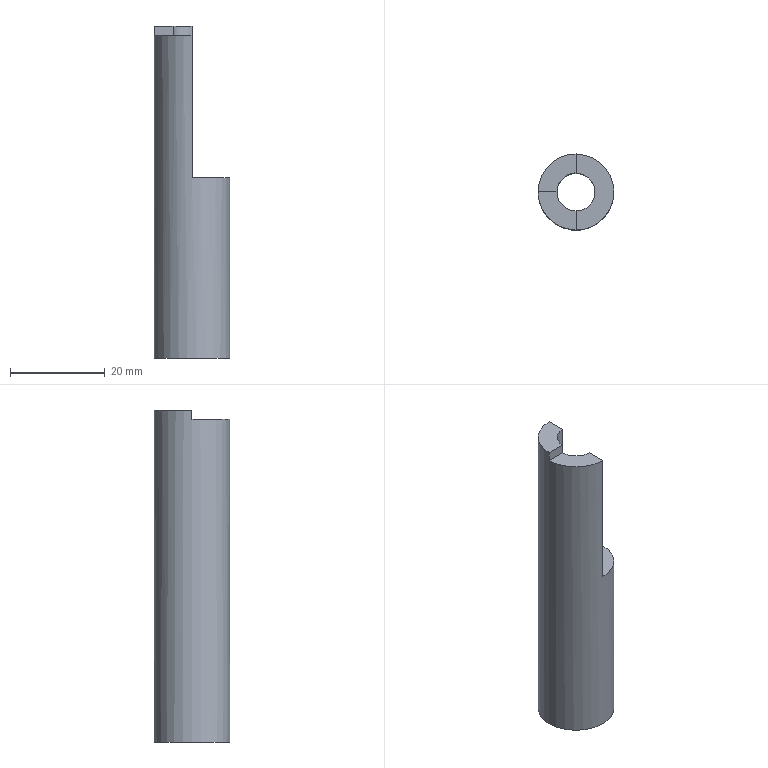Part | NX | features solid 2 | 1 solid | 9 faces | box 16 x 16 x 70 mm | volume 8068 mm3 | plane 7 | cylinder 2 | commonest cylinder face diameters 8 x1 16 x1
STEP:
#1=CARTESIAN_POINT('',(158.,4.,-34.5));
#2=VERTEX_POINT('',#1);
#3=CARTESIAN_POINT('',(158.,8.,-34.5));
#4=VERTEX_POINT('',#3);
#5=CARTESIAN_POINT('',(158.,0.000000002,-34.5));
#6=DIRECTION('',(0.,-1.,0.));
#7=VECTOR('',#6,1000.);
#8=LINE('',#5,#7);
#9=EDGE_CURVE('',#2,#4,#8,.F.);
#10=ORIENTED_EDGE('',*,*,#9,.F.);
#11=CARTESIAN_POINT('',(158.,-4.,-34.5));
#12=VERTEX_POINT('',#11);
#13=CARTESIAN_POINT('',(158.,0.000000002,-34.5));
#14=DIRECTION('',(0.,0.,-1.));
#15=DIRECTION('',(-1.,0.,0.));
#16=AXIS2_PLACEMENT_3D('',#13,#14,#15);
#17=CIRCLE('',#16,4.);
#18=EDGE_CURVE('',#12,#2,#17,.F.);
#19=ORIENTED_EDGE('',*,*,#18,.F.);
#20=CARTESIAN_POINT('',(158.,-8.,-34.5));
#21=VERTEX_POINT('',#20);
#22=CARTESIAN_POINT('',(158.,0.000000002,-34.5));
#23=DIRECTION('',(0.,-1.,0.));
#24=VECTOR('',#23,1000.);
#25=LINE('',#22,#24);
#26=EDGE_CURVE('',#21,#12,#25,.F.);
#27=ORIENTED_EDGE('',*,*,#26,.F.);
#28=CARTESIAN_POINT('',(158.,0.000000002,-34.5));
#29=DIRECTION('',(0.,0.,-1.));
#30=DIRECTION('',(-1.,0.,0.));
#31=AXIS2_PLACEMENT_3D('',#28,#29,#30);
#32=CIRCLE('',#31,8.);
#33=EDGE_CURVE('',#21,#4,#32,.F.);
#34=ORIENTED_EDGE('',*,*,#33,.T.);
#35=EDGE_LOOP('',(#10,#19,#27,#34));
#36=FACE_BOUND('',#35,.T.);
#37=CARTESIAN_POINT('',(158.,0.000000002,-34.5));
#38=DIRECTION('',(0.,0.,-1.));
#39=DIRECTION('',(-1.,0.,0.));
#40=AXIS2_PLACEMENT_3D('',#37,#38,#39);
#41=PLANE('',#40);
#42=ADVANCED_FACE('',(#36),#41,.F.);
#43=ORIENTED_EDGE('',*,*,#18,.T.);
#44=CARTESIAN_POINT('',(158.,4.,-2.5));
#45=VERTEX_POINT('',#44);
#46=CARTESIAN_POINT('',(158.,4.,52.5));
#47=DIRECTION('',(0.,0.,-1.));
#48=VECTOR('',#47,1000.);
#49=LINE('',#46,#48);
#50=EDGE_CURVE('',#45,#2,#49,.T.);
#51=ORIENTED_EDGE('',*,*,#50,.F.);
#52=CARTESIAN_POINT('',(154.,0.000000002,-2.5));
#53=VERTEX_POINT('',#52);
#54=CARTESIAN_POINT('',(158.,0.000000002,-2.5));
#55=DIRECTION('',(0.,0.,1.));
#56=DIRECTION('',(1.,0.,0.));
#57=AXIS2_PLACEMENT_3D('',#54,#55,#56);
#58=CIRCLE('',#57,4.);
#59=EDGE_CURVE('',#53,#45,#58,.F.);
#60=ORIENTED_EDGE('',*,*,#59,.F.);
#61=CARTESIAN_POINT('',(154.,0.000000002,-4.5));
#62=VERTEX_POINT('',#61);
#63=CARTESIAN_POINT('',(154.,0.000000002,52.5));
#64=DIRECTION('',(0.,0.,-1.));
#65=VECTOR('',#64,1000.);
#66=LINE('',#63,#65);
#67=EDGE_CURVE('',#53,#62,#66,.T.);
#68=ORIENTED_EDGE('',*,*,#67,.T.);
#69=CARTESIAN_POINT('',(158.,-4.,-4.5));
#70=VERTEX_POINT('',#69);
#71=CARTESIAN_POINT('',(158.,0.000000002,-4.5));
#72=DIRECTION('',(0.,0.,1.));
#73=DIRECTION('',(1.,0.,0.));
#74=AXIS2_PLACEMENT_3D('',#71,#72,#73);
#75=CIRCLE('',#74,4.);
#76=EDGE_CURVE('',#70,#62,#75,.F.);
#77=ORIENTED_EDGE('',*,*,#76,.F.);
#78=CARTESIAN_POINT('',(158.,-4.,52.5));
#79=DIRECTION('',(0.,0.,-1.));
#80=VECTOR('',#79,1000.);
#81=LINE('',#78,#80);
#82=EDGE_CURVE('',#12,#70,#81,.F.);
#83=ORIENTED_EDGE('',*,*,#82,.F.);
#84=EDGE_LOOP('',(#43,#51,#60,#68,#77,#83));
#85=FACE_BOUND('',#84,.T.);
#86=CARTESIAN_POINT('',(162.,0.000000002,-72.5));
#87=VERTEX_POINT('',#86);
#88=CARTESIAN_POINT('',(158.,0.000000002,-72.5));
#89=DIRECTION('',(0.,0.,1.));
#90=DIRECTION('',(1.,0.,0.));
#91=AXIS2_PLACEMENT_3D('',#88,#89,#90);
#92=CIRCLE('',#91,4.);
#93=EDGE_CURVE('',#87,#87,#92,.T.);
#94=ORIENTED_EDGE('',*,*,#93,.F.);
#95=EDGE_LOOP('',(#94));
#96=FACE_BOUND('',#95,.T.);
#97=CARTESIAN_POINT('',(158.,0.000000002,52.5));
#98=DIRECTION('',(0.,0.,-1.));
#99=DIRECTION('',(-1.,0.,0.));
#100=AXIS2_PLACEMENT_3D('',#97,#98,#99);
#101=CYLINDRICAL_SURFACE('',#100,4.);
#102=ADVANCED_FACE('',(#85,#96),#101,.F.);
#103=ORIENTED_EDGE('',*,*,#33,.F.);
#104=CARTESIAN_POINT('',(158.,-8.,-4.5));
#105=VERTEX_POINT('',#104);
#106=CARTESIAN_POINT('',(158.,-8.,-72.5));
#107=DIRECTION('',(0.,0.,1.));
#108=VECTOR('',#107,1000.);
#109=LINE('',#106,#108);
#110=EDGE_CURVE('',#21,#105,#109,.T.);
#111=ORIENTED_EDGE('',*,*,#110,.T.);
#112=CARTESIAN_POINT('',(150.,0.000000002,-4.5));
#113=VERTEX_POINT('',#112);
#114=CARTESIAN_POINT('',(158.,0.000000002,-4.5));
#115=DIRECTION('',(0.,0.,1.));
#116=DIRECTION('',(1.,0.,0.));
#117=AXIS2_PLACEMENT_3D('',#114,#115,#116);
#118=CIRCLE('',#117,8.);
#119=EDGE_CURVE('',#105,#113,#118,.F.);
#120=ORIENTED_EDGE('',*,*,#119,.T.);
#121=CARTESIAN_POINT('',(150.,0.000000002,-2.5));
#122=VERTEX_POINT('',#121);
#123=CARTESIAN_POINT('',(150.,0.000000002,-72.5));
#124=DIRECTION('',(0.,0.,1.));
#125=VECTOR('',#124,1000.);
#126=LINE('',#123,#125);
#127=EDGE_CURVE('',#122,#113,#126,.F.);
#128=ORIENTED_EDGE('',*,*,#127,.F.);
#129=CARTESIAN_POINT('',(158.,8.,-2.5));
#130=VERTEX_POINT('',#129);
#131=CARTESIAN_POINT('',(158.,0.000000002,-2.5));
#132=DIRECTION('',(0.,0.,1.));
#133=DIRECTION('',(1.,0.,0.));
#134=AXIS2_PLACEMENT_3D('',#131,#132,#133);
#135=CIRCLE('',#134,8.);
#136=EDGE_CURVE('',#122,#130,#135,.F.);
#137=ORIENTED_EDGE('',*,*,#136,.T.);
#138=CARTESIAN_POINT('',(158.,8.,-72.5));
#139=DIRECTION('',(0.,0.,1.));
#140=VECTOR('',#139,1000.);
#141=LINE('',#138,#140);
#142=EDGE_CURVE('',#130,#4,#141,.F.);
#143=ORIENTED_EDGE('',*,*,#142,.T.);
#144=EDGE_LOOP('',(#103,#111,#120,#128,#137,#143));
#145=FACE_BOUND('',#144,.T.);
#146=CARTESIAN_POINT('',(166.,0.000000002,-72.5));
#147=VERTEX_POINT('',#146);
#148=CARTESIAN_POINT('',(158.,0.000000002,-72.5));
#149=DIRECTION('',(0.,0.,1.));
#150=DIRECTION('',(1.,0.,0.));
#151=AXIS2_PLACEMENT_3D('',#148,#149,#150);
#152=CIRCLE('',#151,8.);
#153=EDGE_CURVE('',#147,#147,#152,.T.);
#154=ORIENTED_EDGE('',*,*,#153,.T.);
#155=EDGE_LOOP('',(#154));
#156=FACE_BOUND('',#155,.T.);
#157=CARTESIAN_POINT('',(158.,0.000000002,-72.5));
#158=DIRECTION('',(0.,0.,1.));
#159=DIRECTION('',(1.,0.,0.));
#160=AXIS2_PLACEMENT_3D('',#157,#158,#159);
#161=CYLINDRICAL_SURFACE('',#160,8.);
#162=ADVANCED_FACE('',(#145,#156),#161,.T.);
#163=ORIENTED_EDGE('',*,*,#93,.T.);
#164=EDGE_LOOP('',(#163));
#165=FACE_BOUND('',#164,.T.);
#166=ORIENTED_EDGE('',*,*,#153,.F.);
#167=EDGE_LOOP('',(#166));
#168=FACE_BOUND('',#167,.T.);
#169=CARTESIAN_POINT('',(158.,0.000000002,-72.5));
#170=DIRECTION('',(0.,0.,1.));
#171=DIRECTION('',(1.,0.,0.));
#172=AXIS2_PLACEMENT_3D('',#169,#170,#171);
#173=PLANE('',#172);
#174=ADVANCED_FACE('',(#165,#168),#173,.F.);
#175=ORIENTED_EDGE('',*,*,#26,.T.);
#176=ORIENTED_EDGE('',*,*,#82,.T.);
#177=CARTESIAN_POINT('',(158.,0.000000002,-4.5));
#178=DIRECTION('',(0.,-1.,0.));
#179=VECTOR('',#178,1000.);
#180=LINE('',#177,#179);
#181=EDGE_CURVE('',#70,#105,#180,.T.);
#182=ORIENTED_EDGE('',*,*,#181,.T.);
#183=ORIENTED_EDGE('',*,*,#110,.F.);
#184=EDGE_LOOP('',(#175,#176,#182,#183));
#185=FACE_BOUND('',#184,.T.);
#186=CARTESIAN_POINT('',(158.,0.000000002,-2.5));
#187=DIRECTION('',(1.,0.,0.));
#188=DIRECTION('',(0.,0.,-1.));
#189=AXIS2_PLACEMENT_3D('',#186,#187,#188);
#190=PLANE('',#189);
#191=ADVANCED_FACE('',(#185),#190,.T.);
#192=ORIENTED_EDGE('',*,*,#76,.T.);
#193=CARTESIAN_POINT('',(162.,0.000000002,-4.5));
#194=DIRECTION('',(-1.,0.,0.));
#195=VECTOR('',#194,1000.);
#196=LINE('',#193,#195);
#197=EDGE_CURVE('',#62,#113,#196,.T.);
#198=ORIENTED_EDGE('',*,*,#197,.T.);
#199=ORIENTED_EDGE('',*,*,#119,.F.);
#200=ORIENTED_EDGE('',*,*,#181,.F.);
#201=EDGE_LOOP('',(#192,#198,#199,#200));
#202=FACE_BOUND('',#201,.T.);
#203=CARTESIAN_POINT('',(162.,205.4,-4.5));
#204=DIRECTION('',(0.,0.,1.));
#205=DIRECTION('',(1.,0.,0.));
#206=AXIS2_PLACEMENT_3D('',#203,#204,#205);
#207=PLANE('',#206);
#208=ADVANCED_FACE('',(#202),#207,.T.);
#209=CARTESIAN_POINT('',(162.,0.000000002,-2.5));
#210=DIRECTION('',(-1.,0.,0.));
#211=VECTOR('',#210,1000.);
#212=LINE('',#209,#211);
#213=EDGE_CURVE('',#122,#53,#212,.F.);
#214=ORIENTED_EDGE('',*,*,#213,.T.);
#215=ORIENTED_EDGE('',*,*,#59,.T.);
#216=CARTESIAN_POINT('',(158.,205.4,-2.5));
#217=DIRECTION('',(0.,1.,0.));
#218=VECTOR('',#217,1000.);
#219=LINE('',#216,#218);
#220=EDGE_CURVE('',#130,#45,#219,.F.);
#221=ORIENTED_EDGE('',*,*,#220,.F.);
#222=ORIENTED_EDGE('',*,*,#136,.F.);
#223=EDGE_LOOP('',(#214,#215,#221,#222));
#224=FACE_BOUND('',#223,.T.);
#225=CARTESIAN_POINT('',(162.,205.4,-2.5));
#226=DIRECTION('',(0.,0.,1.));
#227=DIRECTION('',(1.,0.,0.));
#228=AXIS2_PLACEMENT_3D('',#225,#226,#227);
#229=PLANE('',#228);
#230=ADVANCED_FACE('',(#224),#229,.T.);
#231=ORIENTED_EDGE('',*,*,#220,.T.);
#232=ORIENTED_EDGE('',*,*,#50,.T.);
#233=ORIENTED_EDGE('',*,*,#9,.T.);
#234=ORIENTED_EDGE('',*,*,#142,.F.);
#235=EDGE_LOOP('',(#231,#232,#233,#234));
#236=FACE_BOUND('',#235,.T.);
#237=CARTESIAN_POINT('',(158.,0.000000002,-2.5));
#238=DIRECTION('',(1.,0.,0.));
#239=DIRECTION('',(0.,0.,-1.));
#240=AXIS2_PLACEMENT_3D('',#237,#238,#239);
#241=PLANE('',#240);
#242=ADVANCED_FACE('',(#236),#241,.T.);
#243=ORIENTED_EDGE('',*,*,#197,.F.);
#244=ORIENTED_EDGE('',*,*,#67,.F.);
#245=ORIENTED_EDGE('',*,*,#213,.F.);
#246=ORIENTED_EDGE('',*,*,#127,.T.);
#247=EDGE_LOOP('',(#243,#244,#245,#246));
#248=FACE_BOUND('',#247,.T.);
#249=CARTESIAN_POINT('',(158.,0.000000002,-2.5));
#250=DIRECTION('',(0.,1.,0.));
#251=DIRECTION('',(0.,0.,1.));
#252=AXIS2_PLACEMENT_3D('',#249,#250,#251);
#253=PLANE('',#252);
#254=ADVANCED_FACE('',(#248),#253,.F.);
#255=CLOSED_SHELL('',(#42,#102,#162,#174,#191,#208,#230,#242,#254));
#256=MANIFOLD_SOLID_BREP('',#255);
#257=(LENGTH_UNIT()NAMED_UNIT(*)SI_UNIT(.MILLI.,.METRE.));
#258=UNCERTAINTY_MEASURE_WITH_UNIT(LENGTH_MEASURE(0.00001),#257,'','');
#259=(NAMED_UNIT(*)PLANE_ANGLE_UNIT()SI_UNIT($,.RADIAN.));
#260=(NAMED_UNIT(*)SI_UNIT($,.STERADIAN.)SOLID_ANGLE_UNIT());
#261=(GEOMETRIC_REPRESENTATION_CONTEXT(3)GLOBAL_UNCERTAINTY_ASSIGNED_CONTEXT((#258))GLOBAL_UNIT_ASSIGNED_CONTEXT((#257,#259,#260))REPRESENTATION_CONTEXT('',''));
#262=ADVANCED_BREP_SHAPE_REPRESENTATION('',(#256),#261);